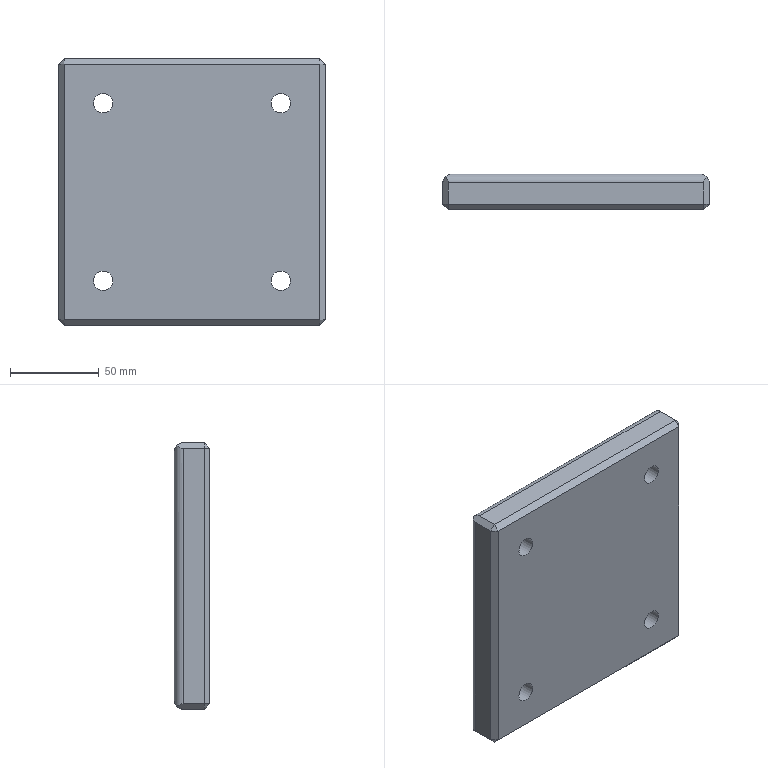Part | NX | features MAIN_BODY 2 | 1 solid | 34 faces | box 150 x 20 x 150 mm | volume 429309 mm3 | plane 22 | cylinder 12 | commonest cylinder face diameters 10 x4 11 x4 17.5 x4
STEP:
#1=CARTESIAN_POINT('',(-692.,520.,325.));
#2=VERTEX_POINT('',#1);
#3=CARTESIAN_POINT('',(-692.,532.,325.));
#4=VERTEX_POINT('',#3);
#5=CARTESIAN_POINT('',(-692.,517.,325.));
#6=DIRECTION('',(0.,1.,0.));
#7=VECTOR('',#6,1000.);
#8=LINE('',#5,#7);
#9=EDGE_CURVE('',#2,#4,#8,.T.);
#10=ORIENTED_EDGE('',*,*,#9,.F.);
#11=CARTESIAN_POINT('',(-548.,520.,325.));
#12=VERTEX_POINT('',#11);
#13=CARTESIAN_POINT('',(-695.,520.,325.));
#14=DIRECTION('',(-1.,0.,0.));
#15=VECTOR('',#14,1000.);
#16=LINE('',#13,#15);
#17=EDGE_CURVE('',#12,#2,#16,.T.);
#18=ORIENTED_EDGE('',*,*,#17,.F.);
#19=CARTESIAN_POINT('',(-548.,532.,325.));
#20=VERTEX_POINT('',#19);
#21=CARTESIAN_POINT('',(-548.,517.,325.));
#22=DIRECTION('',(0.,-1.,0.));
#23=VECTOR('',#22,1000.);
#24=LINE('',#21,#23);
#25=EDGE_CURVE('',#20,#12,#24,.T.);
#26=ORIENTED_EDGE('',*,*,#25,.F.);
#27=CARTESIAN_POINT('',(-548.,532.,325.));
#28=DIRECTION('',(1.,0.,0.));
#29=VECTOR('',#28,1000.);
#30=LINE('',#27,#29);
#31=EDGE_CURVE('',#4,#20,#30,.T.);
#32=ORIENTED_EDGE('',*,*,#31,.F.);
#33=EDGE_LOOP('',(#10,#18,#26,#32));
#34=FACE_BOUND('',#33,.T.);
#35=CARTESIAN_POINT('',(-695.,517.,325.));
#36=DIRECTION('',(0.,0.,-1.));
#37=DIRECTION('',(0.,-1.,0.));
#38=AXIS2_PLACEMENT_3D('',#35,#36,#37);
#39=PLANE('',#38);
#40=ADVANCED_FACE('',(#34),#39,.F.);
#41=CARTESIAN_POINT('',(-545.,520.,322.));
#42=VERTEX_POINT('',#41);
#43=CARTESIAN_POINT('',(-545.,532.,322.));
#44=VERTEX_POINT('',#43);
#45=CARTESIAN_POINT('',(-545.,517.,322.));
#46=DIRECTION('',(0.,1.,0.));
#47=VECTOR('',#46,1000.);
#48=LINE('',#45,#47);
#49=EDGE_CURVE('',#42,#44,#48,.T.);
#50=ORIENTED_EDGE('',*,*,#49,.F.);
#51=CARTESIAN_POINT('',(-545.,520.,178.));
#52=VERTEX_POINT('',#51);
#53=CARTESIAN_POINT('',(-545.,520.,325.));
#54=DIRECTION('',(0.,0.,1.));
#55=VECTOR('',#54,1000.);
#56=LINE('',#53,#55);
#57=EDGE_CURVE('',#52,#42,#56,.T.);
#58=ORIENTED_EDGE('',*,*,#57,.F.);
#59=CARTESIAN_POINT('',(-545.,532.,178.));
#60=VERTEX_POINT('',#59);
#61=CARTESIAN_POINT('',(-545.,517.,178.));
#62=DIRECTION('',(0.,-1.,0.));
#63=VECTOR('',#62,1000.);
#64=LINE('',#61,#63);
#65=EDGE_CURVE('',#60,#52,#64,.T.);
#66=ORIENTED_EDGE('',*,*,#65,.F.);
#67=CARTESIAN_POINT('',(-545.,532.,178.));
#68=DIRECTION('',(0.,0.,-1.));
#69=VECTOR('',#68,1000.);
#70=LINE('',#67,#69);
#71=EDGE_CURVE('',#44,#60,#70,.T.);
#72=ORIENTED_EDGE('',*,*,#71,.F.);
#73=EDGE_LOOP('',(#50,#58,#66,#72));
#74=FACE_BOUND('',#73,.T.);
#75=CARTESIAN_POINT('',(-545.,517.,325.));
#76=DIRECTION('',(-1.,0.,0.));
#77=DIRECTION('',(0.,0.,-1.));
#78=AXIS2_PLACEMENT_3D('',#75,#76,#77);
#79=PLANE('',#78);
#80=ADVANCED_FACE('',(#74),#79,.F.);
#81=CARTESIAN_POINT('',(-548.,520.,175.));
#82=VERTEX_POINT('',#81);
#83=CARTESIAN_POINT('',(-548.,532.,175.));
#84=VERTEX_POINT('',#83);
#85=CARTESIAN_POINT('',(-548.,517.,175.));
#86=DIRECTION('',(0.,1.,0.));
#87=VECTOR('',#86,1000.);
#88=LINE('',#85,#87);
#89=EDGE_CURVE('',#82,#84,#88,.T.);
#90=ORIENTED_EDGE('',*,*,#89,.F.);
#91=CARTESIAN_POINT('',(-692.,520.,175.));
#92=VERTEX_POINT('',#91);
#93=CARTESIAN_POINT('',(-545.,520.,175.));
#94=DIRECTION('',(1.,0.,0.));
#95=VECTOR('',#94,1000.);
#96=LINE('',#93,#95);
#97=EDGE_CURVE('',#92,#82,#96,.T.);
#98=ORIENTED_EDGE('',*,*,#97,.F.);
#99=CARTESIAN_POINT('',(-692.,532.,175.));
#100=VERTEX_POINT('',#99);
#101=CARTESIAN_POINT('',(-692.,517.,175.));
#102=DIRECTION('',(0.,-1.,0.));
#103=VECTOR('',#102,1000.);
#104=LINE('',#101,#103);
#105=EDGE_CURVE('',#100,#92,#104,.T.);
#106=ORIENTED_EDGE('',*,*,#105,.F.);
#107=CARTESIAN_POINT('',(-692.,532.,175.));
#108=DIRECTION('',(-1.,0.,0.));
#109=VECTOR('',#108,1000.);
#110=LINE('',#107,#109);
#111=EDGE_CURVE('',#84,#100,#110,.T.);
#112=ORIENTED_EDGE('',*,*,#111,.F.);
#113=EDGE_LOOP('',(#90,#98,#106,#112));
#114=FACE_BOUND('',#113,.T.);
#115=CARTESIAN_POINT('',(-545.,517.,175.));
#116=DIRECTION('',(0.,0.,1.));
#117=DIRECTION('',(-1.,0.,0.));
#118=AXIS2_PLACEMENT_3D('',#115,#116,#117);
#119=PLANE('',#118);
#120=ADVANCED_FACE('',(#114),#119,.F.);
#121=CARTESIAN_POINT('',(-695.,520.,178.));
#122=VERTEX_POINT('',#121);
#123=CARTESIAN_POINT('',(-695.,532.,178.));
#124=VERTEX_POINT('',#123);
#125=CARTESIAN_POINT('',(-695.,517.,178.));
#126=DIRECTION('',(0.,1.,0.));
#127=VECTOR('',#126,1000.);
#128=LINE('',#125,#127);
#129=EDGE_CURVE('',#122,#124,#128,.T.);
#130=ORIENTED_EDGE('',*,*,#129,.F.);
#131=CARTESIAN_POINT('',(-695.,520.,322.));
#132=VERTEX_POINT('',#131);
#133=CARTESIAN_POINT('',(-695.,520.,175.));
#134=DIRECTION('',(0.,0.,-1.));
#135=VECTOR('',#134,1000.);
#136=LINE('',#133,#135);
#137=EDGE_CURVE('',#132,#122,#136,.T.);
#138=ORIENTED_EDGE('',*,*,#137,.F.);
#139=CARTESIAN_POINT('',(-695.,532.,322.));
#140=VERTEX_POINT('',#139);
#141=CARTESIAN_POINT('',(-695.,517.,322.));
#142=DIRECTION('',(0.,-1.,0.));
#143=VECTOR('',#142,1000.);
#144=LINE('',#141,#143);
#145=EDGE_CURVE('',#140,#132,#144,.T.);
#146=ORIENTED_EDGE('',*,*,#145,.F.);
#147=CARTESIAN_POINT('',(-695.,532.,322.));
#148=DIRECTION('',(0.,0.,1.));
#149=VECTOR('',#148,1000.);
#150=LINE('',#147,#149);
#151=EDGE_CURVE('',#124,#140,#150,.T.);
#152=ORIENTED_EDGE('',*,*,#151,.F.);
#153=EDGE_LOOP('',(#130,#138,#146,#152));
#154=FACE_BOUND('',#153,.T.);
#155=CARTESIAN_POINT('',(-695.,517.,175.));
#156=DIRECTION('',(1.,0.,0.));
#157=DIRECTION('',(0.,0.,1.));
#158=AXIS2_PLACEMENT_3D('',#155,#156,#157);
#159=PLANE('',#158);
#160=ADVANCED_FACE('',(#154),#159,.F.);
#161=CARTESIAN_POINT('',(-692.,517.,178.));
#162=VERTEX_POINT('',#161);
#163=CARTESIAN_POINT('',(-692.,517.,322.));
#164=VERTEX_POINT('',#163);
#165=CARTESIAN_POINT('',(-692.,517.,325.));
#166=DIRECTION('',(0.,0.,1.));
#167=VECTOR('',#166,1000.);
#168=LINE('',#165,#167);
#169=EDGE_CURVE('',#162,#164,#168,.T.);
#170=ORIENTED_EDGE('',*,*,#169,.F.);
#171=CARTESIAN_POINT('',(-548.,517.,178.));
#172=VERTEX_POINT('',#171);
#173=CARTESIAN_POINT('',(-695.,517.,178.));
#174=DIRECTION('',(-1.,0.,0.));
#175=VECTOR('',#174,1000.);
#176=LINE('',#173,#175);
#177=EDGE_CURVE('',#172,#162,#176,.T.);
#178=ORIENTED_EDGE('',*,*,#177,.F.);
#179=CARTESIAN_POINT('',(-548.,517.,322.));
#180=VERTEX_POINT('',#179);
#181=CARTESIAN_POINT('',(-548.,517.,325.));
#182=DIRECTION('',(0.,0.,-1.));
#183=VECTOR('',#182,1000.);
#184=LINE('',#181,#183);
#185=EDGE_CURVE('',#180,#172,#184,.T.);
#186=ORIENTED_EDGE('',*,*,#185,.F.);
#187=CARTESIAN_POINT('',(-695.,517.,322.));
#188=DIRECTION('',(1.,0.,0.));
#189=VECTOR('',#188,1000.);
#190=LINE('',#187,#189);
#191=EDGE_CURVE('',#164,#180,#190,.T.);
#192=ORIENTED_EDGE('',*,*,#191,.F.);
#193=EDGE_LOOP('',(#170,#178,#186,#192));
#194=FACE_BOUND('',#193,.T.);
#195=CARTESIAN_POINT('',(-564.5,517.,300.));
#196=VERTEX_POINT('',#195);
#197=CARTESIAN_POINT('',(-570.,517.,300.));
#198=DIRECTION('',(0.,-1.,0.));
#199=DIRECTION('',(1.,0.,0.));
#200=AXIS2_PLACEMENT_3D('',#197,#198,#199);
#201=CIRCLE('',#200,5.5);
#202=EDGE_CURVE('',#196,#196,#201,.T.);
#203=ORIENTED_EDGE('',*,*,#202,.F.);
#204=EDGE_LOOP('',(#203));
#205=FACE_BOUND('',#204,.T.);
#206=CARTESIAN_POINT('',(-664.5,517.,300.));
#207=VERTEX_POINT('',#206);
#208=CARTESIAN_POINT('',(-670.,517.,300.));
#209=DIRECTION('',(0.,-1.,0.));
#210=DIRECTION('',(1.,0.,0.));
#211=AXIS2_PLACEMENT_3D('',#208,#209,#210);
#212=CIRCLE('',#211,5.5);
#213=EDGE_CURVE('',#207,#207,#212,.T.);
#214=ORIENTED_EDGE('',*,*,#213,.F.);
#215=EDGE_LOOP('',(#214));
#216=FACE_BOUND('',#215,.T.);
#217=CARTESIAN_POINT('',(-664.5,517.,200.));
#218=VERTEX_POINT('',#217);
#219=CARTESIAN_POINT('',(-670.,517.,200.));
#220=DIRECTION('',(0.,-1.,0.));
#221=DIRECTION('',(1.,0.,0.));
#222=AXIS2_PLACEMENT_3D('',#219,#220,#221);
#223=CIRCLE('',#222,5.5);
#224=EDGE_CURVE('',#218,#218,#223,.T.);
#225=ORIENTED_EDGE('',*,*,#224,.F.);
#226=EDGE_LOOP('',(#225));
#227=FACE_BOUND('',#226,.T.);
#228=CARTESIAN_POINT('',(-564.5,517.,200.));
#229=VERTEX_POINT('',#228);
#230=CARTESIAN_POINT('',(-570.,517.,200.));
#231=DIRECTION('',(0.,-1.,0.));
#232=DIRECTION('',(1.,0.,0.));
#233=AXIS2_PLACEMENT_3D('',#230,#231,#232);
#234=CIRCLE('',#233,5.5);
#235=EDGE_CURVE('',#229,#229,#234,.T.);
#236=ORIENTED_EDGE('',*,*,#235,.F.);
#237=EDGE_LOOP('',(#236));
#238=FACE_BOUND('',#237,.T.);
#239=CARTESIAN_POINT('',(-695.,517.,325.));
#240=DIRECTION('',(0.,1.,0.));
#241=DIRECTION('',(1.,0.,0.));
#242=AXIS2_PLACEMENT_3D('',#239,#240,#241);
#243=PLANE('',#242);
#244=ADVANCED_FACE('',(#194,#205,#216,#227,#238),#243,.F.);
#245=CARTESIAN_POINT('',(-690.,537.,180.));
#246=VERTEX_POINT('',#245);
#247=CARTESIAN_POINT('',(-550.,537.,180.));
#248=VERTEX_POINT('',#247);
#249=CARTESIAN_POINT('',(-548.,537.,180.));
#250=DIRECTION('',(-1.,0.,0.));
#251=VECTOR('',#250,1000.);
#252=LINE('',#249,#251);
#253=EDGE_CURVE('',#246,#248,#252,.F.);
#254=ORIENTED_EDGE('',*,*,#253,.F.);
#255=CARTESIAN_POINT('',(-690.,537.,320.));
#256=VERTEX_POINT('',#255);
#257=CARTESIAN_POINT('',(-690.,537.,178.));
#258=DIRECTION('',(0.,0.,1.));
#259=VECTOR('',#258,1000.);
#260=LINE('',#257,#259);
#261=EDGE_CURVE('',#256,#246,#260,.F.);
#262=ORIENTED_EDGE('',*,*,#261,.F.);
#263=CARTESIAN_POINT('',(-550.,537.,320.));
#264=VERTEX_POINT('',#263);
#265=CARTESIAN_POINT('',(-692.,537.,320.));
#266=DIRECTION('',(1.,0.,0.));
#267=VECTOR('',#266,1000.);
#268=LINE('',#265,#267);
#269=EDGE_CURVE('',#264,#256,#268,.F.);
#270=ORIENTED_EDGE('',*,*,#269,.F.);
#271=CARTESIAN_POINT('',(-550.,537.,322.));
#272=DIRECTION('',(0.,0.,-1.));
#273=VECTOR('',#272,1000.);
#274=LINE('',#271,#273);
#275=EDGE_CURVE('',#248,#264,#274,.F.);
#276=ORIENTED_EDGE('',*,*,#275,.F.);
#277=EDGE_LOOP('',(#254,#262,#270,#276));
#278=FACE_BOUND('',#277,.T.);
#279=CARTESIAN_POINT('',(-578.75,537.,300.));
#280=VERTEX_POINT('',#279);
#281=CARTESIAN_POINT('',(-570.,537.,300.));
#282=DIRECTION('',(0.,1.,0.));
#283=DIRECTION('',(-1.,0.,0.));
#284=AXIS2_PLACEMENT_3D('',#281,#282,#283);
#285=CIRCLE('',#284,8.75);
#286=EDGE_CURVE('',#280,#280,#285,.T.);
#287=ORIENTED_EDGE('',*,*,#286,.F.);
#288=EDGE_LOOP('',(#287));
#289=FACE_BOUND('',#288,.T.);
#290=CARTESIAN_POINT('',(-678.75,537.,300.));
#291=VERTEX_POINT('',#290);
#292=CARTESIAN_POINT('',(-670.,537.,300.));
#293=DIRECTION('',(0.,1.,0.));
#294=DIRECTION('',(-1.,0.,0.));
#295=AXIS2_PLACEMENT_3D('',#292,#293,#294);
#296=CIRCLE('',#295,8.75);
#297=EDGE_CURVE('',#291,#291,#296,.T.);
#298=ORIENTED_EDGE('',*,*,#297,.F.);
#299=EDGE_LOOP('',(#298));
#300=FACE_BOUND('',#299,.T.);
#301=CARTESIAN_POINT('',(-678.75,537.,200.));
#302=VERTEX_POINT('',#301);
#303=CARTESIAN_POINT('',(-670.,537.,200.));
#304=DIRECTION('',(0.,1.,0.));
#305=DIRECTION('',(-1.,0.,0.));
#306=AXIS2_PLACEMENT_3D('',#303,#304,#305);
#307=CIRCLE('',#306,8.75);
#308=EDGE_CURVE('',#302,#302,#307,.T.);
#309=ORIENTED_EDGE('',*,*,#308,.F.);
#310=EDGE_LOOP('',(#309));
#311=FACE_BOUND('',#310,.T.);
#312=CARTESIAN_POINT('',(-578.75,537.,200.));
#313=VERTEX_POINT('',#312);
#314=CARTESIAN_POINT('',(-570.,537.,200.));
#315=DIRECTION('',(0.,1.,0.));
#316=DIRECTION('',(-1.,0.,0.));
#317=AXIS2_PLACEMENT_3D('',#314,#315,#316);
#318=CIRCLE('',#317,8.75);
#319=EDGE_CURVE('',#313,#313,#318,.T.);
#320=ORIENTED_EDGE('',*,*,#319,.F.);
#321=EDGE_LOOP('',(#320));
#322=FACE_BOUND('',#321,.T.);
#323=CARTESIAN_POINT('',(-695.,537.,325.));
#324=DIRECTION('',(0.,1.,0.));
#325=DIRECTION('',(1.,0.,0.));
#326=AXIS2_PLACEMENT_3D('',#323,#324,#325);
#327=PLANE('',#326);
#328=ADVANCED_FACE('',(#278,#289,#300,#311,#322),#327,.T.);
#329=CARTESIAN_POINT('',(-575.5,525.,200.));
#330=VERTEX_POINT('',#329);
#331=CARTESIAN_POINT('',(-570.,525.,200.));
#332=DIRECTION('',(0.,1.,0.));
#333=DIRECTION('',(-1.,0.,0.));
#334=AXIS2_PLACEMENT_3D('',#331,#332,#333);
#335=CIRCLE('',#334,5.5);
#336=EDGE_CURVE('',#330,#330,#335,.T.);
#337=ORIENTED_EDGE('',*,*,#336,.T.);
#338=EDGE_LOOP('',(#337));
#339=FACE_BOUND('',#338,.T.);
#340=ORIENTED_EDGE('',*,*,#235,.T.);
#341=EDGE_LOOP('',(#340));
#342=FACE_BOUND('',#341,.T.);
#343=CARTESIAN_POINT('',(-570.,487.,200.));
#344=DIRECTION('',(0.,-1.,0.));
#345=DIRECTION('',(-1.,0.,0.));
#346=AXIS2_PLACEMENT_3D('',#343,#344,#345);
#347=CYLINDRICAL_SURFACE('',#346,5.5);
#348=ADVANCED_FACE('',(#339,#342),#347,.F.);
#349=ORIENTED_EDGE('',*,*,#336,.F.);
#350=EDGE_LOOP('',(#349));
#351=FACE_BOUND('',#350,.T.);
#352=CARTESIAN_POINT('',(-578.75,525.,200.));
#353=VERTEX_POINT('',#352);
#354=CARTESIAN_POINT('',(-570.,525.,200.));
#355=DIRECTION('',(0.,1.,0.));
#356=DIRECTION('',(-1.,0.,0.));
#357=AXIS2_PLACEMENT_3D('',#354,#355,#356);
#358=CIRCLE('',#357,8.75);
#359=EDGE_CURVE('',#353,#353,#358,.T.);
#360=ORIENTED_EDGE('',*,*,#359,.T.);
#361=EDGE_LOOP('',(#360));
#362=FACE_BOUND('',#361,.T.);
#363=CARTESIAN_POINT('',(-570.,525.,200.));
#364=DIRECTION('',(0.,-1.,0.));
#365=DIRECTION('',(-1.,0.,0.));
#366=AXIS2_PLACEMENT_3D('',#363,#364,#365);
#367=PLANE('',#366);
#368=ADVANCED_FACE('',(#351,#362),#367,.F.);
#369=ORIENTED_EDGE('',*,*,#359,.F.);
#370=EDGE_LOOP('',(#369));
#371=FACE_BOUND('',#370,.T.);
#372=ORIENTED_EDGE('',*,*,#319,.T.);
#373=EDGE_LOOP('',(#372));
#374=FACE_BOUND('',#373,.T.);
#375=CARTESIAN_POINT('',(-570.,537.,200.));
#376=DIRECTION('',(0.,-1.,0.));
#377=DIRECTION('',(-1.,0.,0.));
#378=AXIS2_PLACEMENT_3D('',#375,#376,#377);
#379=CYLINDRICAL_SURFACE('',#378,8.75);
#380=ADVANCED_FACE('',(#371,#374),#379,.F.);
#381=CARTESIAN_POINT('',(-675.5,525.,200.));
#382=VERTEX_POINT('',#381);
#383=CARTESIAN_POINT('',(-670.,525.,200.));
#384=DIRECTION('',(0.,1.,0.));
#385=DIRECTION('',(-1.,0.,0.));
#386=AXIS2_PLACEMENT_3D('',#383,#384,#385);
#387=CIRCLE('',#386,5.5);
#388=EDGE_CURVE('',#382,#382,#387,.T.);
#389=ORIENTED_EDGE('',*,*,#388,.T.);
#390=EDGE_LOOP('',(#389));
#391=FACE_BOUND('',#390,.T.);
#392=ORIENTED_EDGE('',*,*,#224,.T.);
#393=EDGE_LOOP('',(#392));
#394=FACE_BOUND('',#393,.T.);
#395=CARTESIAN_POINT('',(-670.,487.,200.));
#396=DIRECTION('',(0.,-1.,0.));
#397=DIRECTION('',(-1.,0.,0.));
#398=AXIS2_PLACEMENT_3D('',#395,#396,#397);
#399=CYLINDRICAL_SURFACE('',#398,5.5);
#400=ADVANCED_FACE('',(#391,#394),#399,.F.);
#401=ORIENTED_EDGE('',*,*,#388,.F.);
#402=EDGE_LOOP('',(#401));
#403=FACE_BOUND('',#402,.T.);
#404=CARTESIAN_POINT('',(-678.75,525.,200.));
#405=VERTEX_POINT('',#404);
#406=CARTESIAN_POINT('',(-670.,525.,200.));
#407=DIRECTION('',(0.,1.,0.));
#408=DIRECTION('',(-1.,0.,0.));
#409=AXIS2_PLACEMENT_3D('',#406,#407,#408);
#410=CIRCLE('',#409,8.75);
#411=EDGE_CURVE('',#405,#405,#410,.T.);
#412=ORIENTED_EDGE('',*,*,#411,.T.);
#413=EDGE_LOOP('',(#412));
#414=FACE_BOUND('',#413,.T.);
#415=CARTESIAN_POINT('',(-670.,525.,200.));
#416=DIRECTION('',(0.,-1.,0.));
#417=DIRECTION('',(-1.,0.,0.));
#418=AXIS2_PLACEMENT_3D('',#415,#416,#417);
#419=PLANE('',#418);
#420=ADVANCED_FACE('',(#403,#414),#419,.F.);
#421=ORIENTED_EDGE('',*,*,#411,.F.);
#422=EDGE_LOOP('',(#421));
#423=FACE_BOUND('',#422,.T.);
#424=ORIENTED_EDGE('',*,*,#308,.T.);
#425=EDGE_LOOP('',(#424));
#426=FACE_BOUND('',#425,.T.);
#427=CARTESIAN_POINT('',(-670.,537.,200.));
#428=DIRECTION('',(0.,-1.,0.));
#429=DIRECTION('',(-1.,0.,0.));
#430=AXIS2_PLACEMENT_3D('',#427,#428,#429);
#431=CYLINDRICAL_SURFACE('',#430,8.75);
#432=ADVANCED_FACE('',(#423,#426),#431,.F.);
#433=CARTESIAN_POINT('',(-675.5,525.,300.));
#434=VERTEX_POINT('',#433);
#435=CARTESIAN_POINT('',(-670.,525.,300.));
#436=DIRECTION('',(0.,1.,0.));
#437=DIRECTION('',(-1.,0.,0.));
#438=AXIS2_PLACEMENT_3D('',#435,#436,#437);
#439=CIRCLE('',#438,5.5);
#440=EDGE_CURVE('',#434,#434,#439,.T.);
#441=ORIENTED_EDGE('',*,*,#440,.T.);
#442=EDGE_LOOP('',(#441));
#443=FACE_BOUND('',#442,.T.);
#444=ORIENTED_EDGE('',*,*,#213,.T.);
#445=EDGE_LOOP('',(#444));
#446=FACE_BOUND('',#445,.T.);
#447=CARTESIAN_POINT('',(-670.,487.,300.));
#448=DIRECTION('',(0.,-1.,0.));
#449=DIRECTION('',(-1.,0.,0.));
#450=AXIS2_PLACEMENT_3D('',#447,#448,#449);
#451=CYLINDRICAL_SURFACE('',#450,5.5);
#452=ADVANCED_FACE('',(#443,#446),#451,.F.);
#453=ORIENTED_EDGE('',*,*,#440,.F.);
#454=EDGE_LOOP('',(#453));
#455=FACE_BOUND('',#454,.T.);
#456=CARTESIAN_POINT('',(-678.75,525.,300.));
#457=VERTEX_POINT('',#456);
#458=CARTESIAN_POINT('',(-670.,525.,300.));
#459=DIRECTION('',(0.,1.,0.));
#460=DIRECTION('',(-1.,0.,0.));
#461=AXIS2_PLACEMENT_3D('',#458,#459,#460);
#462=CIRCLE('',#461,8.75);
#463=EDGE_CURVE('',#457,#457,#462,.T.);
#464=ORIENTED_EDGE('',*,*,#463,.T.);
#465=EDGE_LOOP('',(#464));
#466=FACE_BOUND('',#465,.T.);
#467=CARTESIAN_POINT('',(-670.,525.,300.));
#468=DIRECTION('',(0.,-1.,0.));
#469=DIRECTION('',(-1.,0.,0.));
#470=AXIS2_PLACEMENT_3D('',#467,#468,#469);
#471=PLANE('',#470);
#472=ADVANCED_FACE('',(#455,#466),#471,.F.);
#473=ORIENTED_EDGE('',*,*,#463,.F.);
#474=EDGE_LOOP('',(#473));
#475=FACE_BOUND('',#474,.T.);
#476=ORIENTED_EDGE('',*,*,#297,.T.);
#477=EDGE_LOOP('',(#476));
#478=FACE_BOUND('',#477,.T.);
#479=CARTESIAN_POINT('',(-670.,537.,300.));
#480=DIRECTION('',(0.,-1.,0.));
#481=DIRECTION('',(-1.,0.,0.));
#482=AXIS2_PLACEMENT_3D('',#479,#480,#481);
#483=CYLINDRICAL_SURFACE('',#482,8.75);
#484=ADVANCED_FACE('',(#475,#478),#483,.F.);
#485=CARTESIAN_POINT('',(-575.5,525.,300.));
#486=VERTEX_POINT('',#485);
#487=CARTESIAN_POINT('',(-570.,525.,300.));
#488=DIRECTION('',(0.,1.,0.));
#489=DIRECTION('',(-1.,0.,0.));
#490=AXIS2_PLACEMENT_3D('',#487,#488,#489);
#491=CIRCLE('',#490,5.5);
#492=EDGE_CURVE('',#486,#486,#491,.T.);
#493=ORIENTED_EDGE('',*,*,#492,.T.);
#494=EDGE_LOOP('',(#493));
#495=FACE_BOUND('',#494,.T.);
#496=ORIENTED_EDGE('',*,*,#202,.T.);
#497=EDGE_LOOP('',(#496));
#498=FACE_BOUND('',#497,.T.);
#499=CARTESIAN_POINT('',(-570.,487.,300.));
#500=DIRECTION('',(0.,-1.,0.));
#501=DIRECTION('',(-1.,0.,0.));
#502=AXIS2_PLACEMENT_3D('',#499,#500,#501);
#503=CYLINDRICAL_SURFACE('',#502,5.5);
#504=ADVANCED_FACE('',(#495,#498),#503,.F.);
#505=ORIENTED_EDGE('',*,*,#492,.F.);
#506=EDGE_LOOP('',(#505));
#507=FACE_BOUND('',#506,.T.);
#508=CARTESIAN_POINT('',(-578.75,525.,300.));
#509=VERTEX_POINT('',#508);
#510=CARTESIAN_POINT('',(-570.,525.,300.));
#511=DIRECTION('',(0.,1.,0.));
#512=DIRECTION('',(-1.,0.,0.));
#513=AXIS2_PLACEMENT_3D('',#510,#511,#512);
#514=CIRCLE('',#513,8.75);
#515=EDGE_CURVE('',#509,#509,#514,.T.);
#516=ORIENTED_EDGE('',*,*,#515,.T.);
#517=EDGE_LOOP('',(#516));
#518=FACE_BOUND('',#517,.T.);
#519=CARTESIAN_POINT('',(-570.,525.,300.));
#520=DIRECTION('',(0.,-1.,0.));
#521=DIRECTION('',(-1.,0.,0.));
#522=AXIS2_PLACEMENT_3D('',#519,#520,#521);
#523=PLANE('',#522);
#524=ADVANCED_FACE('',(#507,#518),#523,.F.);
#525=ORIENTED_EDGE('',*,*,#515,.F.);
#526=EDGE_LOOP('',(#525));
#527=FACE_BOUND('',#526,.T.);
#528=ORIENTED_EDGE('',*,*,#286,.T.);
#529=EDGE_LOOP('',(#528));
#530=FACE_BOUND('',#529,.T.);
#531=CARTESIAN_POINT('',(-570.,537.,300.));
#532=DIRECTION('',(0.,-1.,0.));
#533=DIRECTION('',(-1.,0.,0.));
#534=AXIS2_PLACEMENT_3D('',#531,#532,#533);
#535=CYLINDRICAL_SURFACE('',#534,8.75);
#536=ADVANCED_FACE('',(#527,#530),#535,.F.);
#537=CARTESIAN_POINT('',(-693.5,535.571,176.5));
#538=VERTEX_POINT('',#537);
#539=CARTESIAN_POINT('',(-697.,532.,180.));
#540=DIRECTION('',(-0.7071,0.,-0.7071));
#541=DIRECTION('',(0.7071,0.,-0.7071));
#542=AXIS2_PLACEMENT_3D('',#539,#540,#541);
#543=ELLIPSE('',#542,7.071,5.);
#544=EDGE_CURVE('',#100,#538,#543,.F.);
#545=ORIENTED_EDGE('',*,*,#544,.F.);
#546=ORIENTED_EDGE('',*,*,#105,.T.);
#547=CARTESIAN_POINT('',(-695.,520.,178.));
#548=DIRECTION('',(0.7071,0.,-0.7071));
#549=VECTOR('',#548,1000.);
#550=LINE('',#547,#549);
#551=EDGE_CURVE('',#92,#122,#550,.F.);
#552=ORIENTED_EDGE('',*,*,#551,.T.);
#553=ORIENTED_EDGE('',*,*,#129,.T.);
#554=CARTESIAN_POINT('',(-690.,532.,173.));
#555=DIRECTION('',(-0.7071,0.,-0.7071));
#556=DIRECTION('',(0.7071,0.,-0.7071));
#557=AXIS2_PLACEMENT_3D('',#554,#555,#556);
#558=ELLIPSE('',#557,7.071,5.);
#559=EDGE_CURVE('',#538,#124,#558,.F.);
#560=ORIENTED_EDGE('',*,*,#559,.F.);
#561=EDGE_LOOP('',(#545,#546,#552,#553,#560));
#562=FACE_BOUND('',#561,.T.);
#563=CARTESIAN_POINT('',(-695.,517.,178.));
#564=DIRECTION('',(0.7071,0.,0.7071));
#565=DIRECTION('',(-0.7071,0.,0.7071));
#566=AXIS2_PLACEMENT_3D('',#563,#564,#565);
#567=PLANE('',#566);
#568=ADVANCED_FACE('',(#562),#567,.F.);
#569=CARTESIAN_POINT('',(-548.,520.,175.));
#570=DIRECTION('',(0.,0.7071,-0.7071));
#571=VECTOR('',#570,1000.);
#572=LINE('',#569,#571);
#573=EDGE_CURVE('',#82,#172,#572,.F.);
#574=ORIENTED_EDGE('',*,*,#573,.T.);
#575=ORIENTED_EDGE('',*,*,#177,.T.);
#576=CARTESIAN_POINT('',(-692.,518.5,176.5));
#577=DIRECTION('',(0.,-0.7071,0.7071));
#578=VECTOR('',#577,1000.);
#579=LINE('',#576,#578);
#580=EDGE_CURVE('',#162,#92,#579,.F.);
#581=ORIENTED_EDGE('',*,*,#580,.T.);
#582=ORIENTED_EDGE('',*,*,#97,.T.);
#583=EDGE_LOOP('',(#574,#575,#581,#582));
#584=FACE_BOUND('',#583,.T.);
#585=CARTESIAN_POINT('',(-695.,517.,178.));
#586=DIRECTION('',(0.,0.7071,0.7071));
#587=DIRECTION('',(0.,0.7071,-0.7071));
#588=AXIS2_PLACEMENT_3D('',#585,#586,#587);
#589=PLANE('',#588);
#590=ADVANCED_FACE('',(#584),#589,.F.);
#591=ORIENTED_EDGE('',*,*,#65,.T.);
#592=CARTESIAN_POINT('',(-548.,520.,175.));
#593=DIRECTION('',(0.7071,0.,0.7071));
#594=VECTOR('',#593,1000.);
#595=LINE('',#592,#594);
#596=EDGE_CURVE('',#52,#82,#595,.F.);
#597=ORIENTED_EDGE('',*,*,#596,.T.);
#598=ORIENTED_EDGE('',*,*,#89,.T.);
#599=CARTESIAN_POINT('',(-546.5,535.571,176.5));
#600=VERTEX_POINT('',#599);
#601=CARTESIAN_POINT('',(-543.,532.,180.));
#602=DIRECTION('',(0.7071,0.,-0.7071));
#603=DIRECTION('',(0.7071,0.,0.7071));
#604=AXIS2_PLACEMENT_3D('',#601,#602,#603);
#605=ELLIPSE('',#604,7.071,5.);
#606=EDGE_CURVE('',#600,#84,#605,.F.);
#607=ORIENTED_EDGE('',*,*,#606,.F.);
#608=CARTESIAN_POINT('',(-550.,532.,173.));
#609=DIRECTION('',(0.7071,0.,-0.7071));
#610=DIRECTION('',(0.7071,0.,0.7071));
#611=AXIS2_PLACEMENT_3D('',#608,#609,#610);
#612=ELLIPSE('',#611,7.071,5.);
#613=EDGE_CURVE('',#60,#600,#612,.F.);
#614=ORIENTED_EDGE('',*,*,#613,.F.);
#615=EDGE_LOOP('',(#591,#597,#598,#607,#614));
#616=FACE_BOUND('',#615,.T.);
#617=CARTESIAN_POINT('',(-548.,517.,175.));
#618=DIRECTION('',(-0.7071,0.,0.7071));
#619=DIRECTION('',(-0.7071,0.,-0.7071));
#620=AXIS2_PLACEMENT_3D('',#617,#618,#619);
#621=PLANE('',#620);
#622=ADVANCED_FACE('',(#616),#621,.F.);
#623=ORIENTED_EDGE('',*,*,#580,.F.);
#624=CARTESIAN_POINT('',(-695.,520.,178.));
#625=DIRECTION('',(-0.7071,0.7071,0.));
#626=VECTOR('',#625,1000.);
#627=LINE('',#624,#626);
#628=EDGE_CURVE('',#162,#122,#627,.T.);
#629=ORIENTED_EDGE('',*,*,#628,.T.);
#630=ORIENTED_EDGE('',*,*,#551,.F.);
#631=EDGE_LOOP('',(#623,#629,#630));
#632=FACE_BOUND('',#631,.T.);
#633=CARTESIAN_POINT('',(-695.,520.,178.));
#634=DIRECTION('',(-0.5774,-0.5774,-0.5774));
#635=DIRECTION('',(-0.7071,0.7071,0.));
#636=AXIS2_PLACEMENT_3D('',#633,#634,#635);
#637=PLANE('',#636);
#638=ADVANCED_FACE('',(#632),#637,.T.);
#639=ORIENTED_EDGE('',*,*,#596,.F.);
#640=CARTESIAN_POINT('',(-546.5,518.5,178.));
#641=DIRECTION('',(-0.7071,-0.7071,0.));
#642=VECTOR('',#641,1000.);
#643=LINE('',#640,#642);
#644=EDGE_CURVE('',#52,#172,#643,.T.);
#645=ORIENTED_EDGE('',*,*,#644,.T.);
#646=ORIENTED_EDGE('',*,*,#573,.F.);
#647=EDGE_LOOP('',(#639,#645,#646));
#648=FACE_BOUND('',#647,.T.);
#649=CARTESIAN_POINT('',(-548.,520.,175.));
#650=DIRECTION('',(0.5774,-0.5774,-0.5774));
#651=DIRECTION('',(0.7071,0.,0.7071));
#652=AXIS2_PLACEMENT_3D('',#649,#650,#651);
#653=PLANE('',#652);
#654=ADVANCED_FACE('',(#648),#653,.T.);
#655=CARTESIAN_POINT('',(-693.5,535.571,323.5));
#656=VERTEX_POINT('',#655);
#657=CARTESIAN_POINT('',(-690.,532.,327.));
#658=DIRECTION('',(-0.7071,0.,0.7071));
#659=DIRECTION('',(-0.7071,0.,-0.7071));
#660=AXIS2_PLACEMENT_3D('',#657,#658,#659);
#661=ELLIPSE('',#660,7.071,5.);
#662=EDGE_CURVE('',#140,#656,#661,.F.);
#663=ORIENTED_EDGE('',*,*,#662,.F.);
#664=ORIENTED_EDGE('',*,*,#145,.T.);
#665=CARTESIAN_POINT('',(-692.,520.,325.));
#666=DIRECTION('',(-0.7071,0.,-0.7071));
#667=VECTOR('',#666,1000.);
#668=LINE('',#665,#667);
#669=EDGE_CURVE('',#132,#2,#668,.F.);
#670=ORIENTED_EDGE('',*,*,#669,.T.);
#671=ORIENTED_EDGE('',*,*,#9,.T.);
#672=CARTESIAN_POINT('',(-697.,532.,320.));
#673=DIRECTION('',(-0.7071,0.,0.7071));
#674=DIRECTION('',(-0.7071,0.,-0.7071));
#675=AXIS2_PLACEMENT_3D('',#672,#673,#674);
#676=ELLIPSE('',#675,7.071,5.);
#677=EDGE_CURVE('',#656,#4,#676,.F.);
#678=ORIENTED_EDGE('',*,*,#677,.F.);
#679=EDGE_LOOP('',(#663,#664,#670,#671,#678));
#680=FACE_BOUND('',#679,.T.);
#681=CARTESIAN_POINT('',(-692.,517.,325.));
#682=DIRECTION('',(0.7071,0.,-0.7071));
#683=DIRECTION('',(0.7071,0.,0.7071));
#684=AXIS2_PLACEMENT_3D('',#681,#682,#683);
#685=PLANE('',#684);
#686=ADVANCED_FACE('',(#680),#685,.F.);
#687=ORIENTED_EDGE('',*,*,#628,.F.);
#688=ORIENTED_EDGE('',*,*,#169,.T.);
#689=CARTESIAN_POINT('',(-693.5,518.5,322.));
#690=DIRECTION('',(0.7071,-0.7071,0.));
#691=VECTOR('',#690,1000.);
#692=LINE('',#689,#691);
#693=EDGE_CURVE('',#164,#132,#692,.F.);
#694=ORIENTED_EDGE('',*,*,#693,.T.);
#695=ORIENTED_EDGE('',*,*,#137,.T.);
#696=EDGE_LOOP('',(#687,#688,#694,#695));
#697=FACE_BOUND('',#696,.T.);
#698=CARTESIAN_POINT('',(-692.,517.,325.));
#699=DIRECTION('',(0.7071,0.7071,0.));
#700=DIRECTION('',(0.7071,-0.7071,0.));
#701=AXIS2_PLACEMENT_3D('',#698,#699,#700);
#702=PLANE('',#701);
#703=ADVANCED_FACE('',(#697),#702,.F.);
#704=ORIENTED_EDGE('',*,*,#644,.F.);
#705=ORIENTED_EDGE('',*,*,#57,.T.);
#706=CARTESIAN_POINT('',(-548.,517.,322.));
#707=DIRECTION('',(0.7071,0.7071,0.));
#708=VECTOR('',#707,1000.);
#709=LINE('',#706,#708);
#710=EDGE_CURVE('',#42,#180,#709,.F.);
#711=ORIENTED_EDGE('',*,*,#710,.T.);
#712=ORIENTED_EDGE('',*,*,#185,.T.);
#713=EDGE_LOOP('',(#704,#705,#711,#712));
#714=FACE_BOUND('',#713,.T.);
#715=CARTESIAN_POINT('',(-548.,517.,325.));
#716=DIRECTION('',(-0.7071,0.7071,0.));
#717=DIRECTION('',(0.7071,0.7071,0.));
#718=AXIS2_PLACEMENT_3D('',#715,#716,#717);
#719=PLANE('',#718);
#720=ADVANCED_FACE('',(#714),#719,.F.);
#721=CARTESIAN_POINT('',(-546.5,535.571,323.5));
#722=VERTEX_POINT('',#721);
#723=CARTESIAN_POINT('',(-543.,532.,320.));
#724=DIRECTION('',(0.7071,0.,0.7071));
#725=DIRECTION('',(-0.7071,0.,0.7071));
#726=AXIS2_PLACEMENT_3D('',#723,#724,#725);
#727=ELLIPSE('',#726,7.071,5.);
#728=EDGE_CURVE('',#20,#722,#727,.F.);
#729=ORIENTED_EDGE('',*,*,#728,.F.);
#730=ORIENTED_EDGE('',*,*,#25,.T.);
#731=CARTESIAN_POINT('',(-546.5,520.,323.5));
#732=DIRECTION('',(-0.7071,0.,0.7071));
#733=VECTOR('',#732,1000.);
#734=LINE('',#731,#733);
#735=EDGE_CURVE('',#12,#42,#734,.F.);
#736=ORIENTED_EDGE('',*,*,#735,.T.);
#737=ORIENTED_EDGE('',*,*,#49,.T.);
#738=CARTESIAN_POINT('',(-550.,532.,327.));
#739=DIRECTION('',(0.7071,0.,0.7071));
#740=DIRECTION('',(-0.7071,0.,0.7071));
#741=AXIS2_PLACEMENT_3D('',#738,#739,#740);
#742=ELLIPSE('',#741,7.071,5.);
#743=EDGE_CURVE('',#722,#44,#742,.F.);
#744=ORIENTED_EDGE('',*,*,#743,.F.);
#745=EDGE_LOOP('',(#729,#730,#736,#737,#744));
#746=FACE_BOUND('',#745,.T.);
#747=CARTESIAN_POINT('',(-545.,517.,322.));
#748=DIRECTION('',(-0.7071,0.,-0.7071));
#749=DIRECTION('',(0.7071,0.,-0.7071));
#750=AXIS2_PLACEMENT_3D('',#747,#748,#749);
#751=PLANE('',#750);
#752=ADVANCED_FACE('',(#746),#751,.F.);
#753=ORIENTED_EDGE('',*,*,#693,.F.);
#754=CARTESIAN_POINT('',(-692.,520.,325.));
#755=DIRECTION('',(0.,0.7071,0.7071));
#756=VECTOR('',#755,1000.);
#757=LINE('',#754,#756);
#758=EDGE_CURVE('',#164,#2,#757,.T.);
#759=ORIENTED_EDGE('',*,*,#758,.T.);
#760=ORIENTED_EDGE('',*,*,#669,.F.);
#761=EDGE_LOOP('',(#753,#759,#760));
#762=FACE_BOUND('',#761,.T.);
#763=CARTESIAN_POINT('',(-692.,520.,325.));
#764=DIRECTION('',(-0.5774,-0.5774,0.5774));
#765=DIRECTION('',(-0.7071,0.7071,0.));
#766=AXIS2_PLACEMENT_3D('',#763,#764,#765);
#767=PLANE('',#766);
#768=ADVANCED_FACE('',(#762),#767,.T.);
#769=ORIENTED_EDGE('',*,*,#735,.F.);
#770=CARTESIAN_POINT('',(-548.,517.,322.));
#771=DIRECTION('',(0.,-0.7071,-0.7071));
#772=VECTOR('',#771,1000.);
#773=LINE('',#770,#772);
#774=EDGE_CURVE('',#12,#180,#773,.T.);
#775=ORIENTED_EDGE('',*,*,#774,.T.);
#776=ORIENTED_EDGE('',*,*,#710,.F.);
#777=EDGE_LOOP('',(#769,#775,#776));
#778=FACE_BOUND('',#777,.T.);
#779=CARTESIAN_POINT('',(-548.,517.,322.));
#780=DIRECTION('',(0.5774,-0.5774,0.5774));
#781=DIRECTION('',(-0.7071,0.,0.7071));
#782=AXIS2_PLACEMENT_3D('',#779,#780,#781);
#783=PLANE('',#782);
#784=ADVANCED_FACE('',(#778),#783,.T.);
#785=ORIENTED_EDGE('',*,*,#758,.F.);
#786=ORIENTED_EDGE('',*,*,#191,.T.);
#787=ORIENTED_EDGE('',*,*,#774,.F.);
#788=ORIENTED_EDGE('',*,*,#17,.T.);
#789=EDGE_LOOP('',(#785,#786,#787,#788));
#790=FACE_BOUND('',#789,.T.);
#791=CARTESIAN_POINT('',(-695.,517.,322.));
#792=DIRECTION('',(0.,0.7071,-0.7071));
#793=DIRECTION('',(0.,-0.7071,-0.7071));
#794=AXIS2_PLACEMENT_3D('',#791,#792,#793);
#795=PLANE('',#794);
#796=ADVANCED_FACE('',(#790),#795,.F.);
#797=CARTESIAN_POINT('',(-690.,532.,180.));
#798=DIRECTION('',(-0.7071,0.,0.7071));
#799=DIRECTION('',(0.7071,0.,0.7071));
#800=AXIS2_PLACEMENT_3D('',#797,#798,#799);
#801=ELLIPSE('',#800,7.071,5.);
#802=EDGE_CURVE('',#246,#538,#801,.T.);
#803=ORIENTED_EDGE('',*,*,#802,.T.);
#804=ORIENTED_EDGE('',*,*,#559,.T.);
#805=ORIENTED_EDGE('',*,*,#151,.T.);
#806=ORIENTED_EDGE('',*,*,#662,.T.);
#807=CARTESIAN_POINT('',(-690.,532.,320.));
#808=DIRECTION('',(0.7071,0.,0.7071));
#809=DIRECTION('',(0.7071,0.,-0.7071));
#810=AXIS2_PLACEMENT_3D('',#807,#808,#809);
#811=ELLIPSE('',#810,7.071,5.);
#812=EDGE_CURVE('',#656,#256,#811,.F.);
#813=ORIENTED_EDGE('',*,*,#812,.T.);
#814=ORIENTED_EDGE('',*,*,#261,.T.);
#815=EDGE_LOOP('',(#803,#804,#805,#806,#813,#814));
#816=FACE_BOUND('',#815,.T.);
#817=CARTESIAN_POINT('',(-690.,532.,175.));
#818=DIRECTION('',(0.,0.,-1.));
#819=DIRECTION('',(1.,0.,0.));
#820=AXIS2_PLACEMENT_3D('',#817,#818,#819);
#821=CYLINDRICAL_SURFACE('',#820,5.);
#822=ADVANCED_FACE('',(#816),#821,.T.);
#823=ORIENTED_EDGE('',*,*,#812,.F.);
#824=ORIENTED_EDGE('',*,*,#677,.T.);
#825=ORIENTED_EDGE('',*,*,#31,.T.);
#826=ORIENTED_EDGE('',*,*,#728,.T.);
#827=CARTESIAN_POINT('',(-550.,532.,320.));
#828=DIRECTION('',(0.7071,0.,-0.7071));
#829=DIRECTION('',(-0.7071,0.,-0.7071));
#830=AXIS2_PLACEMENT_3D('',#827,#828,#829);
#831=ELLIPSE('',#830,7.071,5.);
#832=EDGE_CURVE('',#722,#264,#831,.F.);
#833=ORIENTED_EDGE('',*,*,#832,.T.);
#834=ORIENTED_EDGE('',*,*,#269,.T.);
#835=EDGE_LOOP('',(#823,#824,#825,#826,#833,#834));
#836=FACE_BOUND('',#835,.T.);
#837=CARTESIAN_POINT('',(-695.,532.,320.));
#838=DIRECTION('',(-1.,0.,0.));
#839=DIRECTION('',(0.,1.,0.));
#840=AXIS2_PLACEMENT_3D('',#837,#838,#839);
#841=CYLINDRICAL_SURFACE('',#840,5.);
#842=ADVANCED_FACE('',(#836),#841,.T.);
#843=ORIENTED_EDGE('',*,*,#111,.T.);
#844=ORIENTED_EDGE('',*,*,#544,.T.);
#845=ORIENTED_EDGE('',*,*,#802,.F.);
#846=ORIENTED_EDGE('',*,*,#253,.T.);
#847=CARTESIAN_POINT('',(-550.,532.,180.));
#848=DIRECTION('',(-0.7071,0.,-0.7071));
#849=DIRECTION('',(-0.7071,0.,0.7071));
#850=AXIS2_PLACEMENT_3D('',#847,#848,#849);
#851=ELLIPSE('',#850,7.071,5.);
#852=EDGE_CURVE('',#248,#600,#851,.T.);
#853=ORIENTED_EDGE('',*,*,#852,.T.);
#854=ORIENTED_EDGE('',*,*,#606,.T.);
#855=EDGE_LOOP('',(#843,#844,#845,#846,#853,#854));
#856=FACE_BOUND('',#855,.T.);
#857=CARTESIAN_POINT('',(-545.,532.,180.));
#858=DIRECTION('',(1.,0.,0.));
#859=DIRECTION('',(0.,0.,1.));
#860=AXIS2_PLACEMENT_3D('',#857,#858,#859);
#861=CYLINDRICAL_SURFACE('',#860,5.);
#862=ADVANCED_FACE('',(#856),#861,.T.);
#863=ORIENTED_EDGE('',*,*,#832,.F.);
#864=ORIENTED_EDGE('',*,*,#743,.T.);
#865=ORIENTED_EDGE('',*,*,#71,.T.);
#866=ORIENTED_EDGE('',*,*,#613,.T.);
#867=ORIENTED_EDGE('',*,*,#852,.F.);
#868=ORIENTED_EDGE('',*,*,#275,.T.);
#869=EDGE_LOOP('',(#863,#864,#865,#866,#867,#868));
#870=FACE_BOUND('',#869,.T.);
#871=CARTESIAN_POINT('',(-550.,532.,325.));
#872=DIRECTION('',(0.,0.,1.));
#873=DIRECTION('',(-1.,0.,0.));
#874=AXIS2_PLACEMENT_3D('',#871,#872,#873);
#875=CYLINDRICAL_SURFACE('',#874,5.);
#876=ADVANCED_FACE('',(#870),#875,.T.);
#877=CLOSED_SHELL('',(#40,#80,#120,#160,#244,#328,#348,#368,#380,#400,#420,#432,#452,#472,#484,#504,#524,#536,#568,#590,#622,#638,#654,#686,#703,#720,#752,#768,#784,#796,#822,#842,#862,#876));
#878=MANIFOLD_SOLID_BREP('',#877);
#879=(LENGTH_UNIT()NAMED_UNIT(*)SI_UNIT(.MILLI.,.METRE.));
#880=UNCERTAINTY_MEASURE_WITH_UNIT(LENGTH_MEASURE(0.00001),#879,'','');
#881=(NAMED_UNIT(*)PLANE_ANGLE_UNIT()SI_UNIT($,.RADIAN.));
#882=(NAMED_UNIT(*)SI_UNIT($,.STERADIAN.)SOLID_ANGLE_UNIT());
#883=(GEOMETRIC_REPRESENTATION_CONTEXT(3)GLOBAL_UNCERTAINTY_ASSIGNED_CONTEXT((#880))GLOBAL_UNIT_ASSIGNED_CONTEXT((#879,#881,#882))REPRESENTATION_CONTEXT('',''));
#884=ADVANCED_BREP_SHAPE_REPRESENTATION('',(#878),#883);